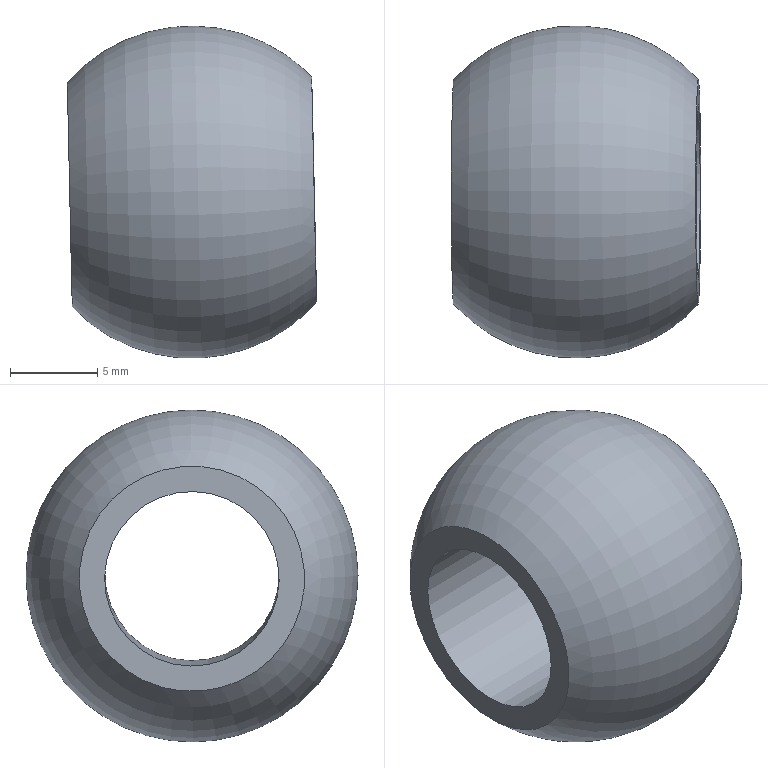Part | NX | features 2 2 | 1 solid | 4 faces | box 14.279 x 19.031 x 19.031 mm | volume 2165 mm3 | plane 2 | cylinder 1 | torus 1 | commonest cylinder face diameters 10 x1
STEP:
#1=CARTESIAN_POINT('',(11.562,55.788,-650.48));
#2=VERTEX_POINT('',#1);
#3=CARTESIAN_POINT('',(11.498,51.587,-647.769));
#4=DIRECTION('',(-0.9998,0.0009413,-0.0219));
#5=DIRECTION('',(0.01267,0.8402,-0.5422));
#6=AXIS2_PLACEMENT_3D('',#3,#4,#5);
#7=CIRCLE('',#6,5.);
#8=EDGE_CURVE('',#2,#2,#7,.T.);
#9=ORIENTED_EDGE('',*,*,#8,.F.);
#10=EDGE_LOOP('',(#9));
#11=FACE_BOUND('',#10,.T.);
#12=CARTESIAN_POINT('',(-2.435,55.801,-650.786));
#13=VERTEX_POINT('',#12);
#14=CARTESIAN_POINT('',(-2.498,51.6,-648.076));
#15=DIRECTION('',(0.9998,-0.0009413,0.0219));
#16=DIRECTION('',(0.01267,0.8402,-0.5422));
#17=AXIS2_PLACEMENT_3D('',#14,#15,#16);
#18=CIRCLE('',#17,5.);
#19=EDGE_CURVE('',#13,#13,#18,.T.);
#20=ORIENTED_EDGE('',*,*,#19,.F.);
#21=EDGE_LOOP('',(#20));
#22=FACE_BOUND('',#21,.T.);
#23=CARTESIAN_POINT('',(4.5,51.593,-647.922));
#24=DIRECTION('',(-0.9998,0.0009413,-0.0219));
#25=DIRECTION('',(0.01267,0.8402,-0.5422));
#26=AXIS2_PLACEMENT_3D('',#23,#24,#25);
#27=CYLINDRICAL_SURFACE('',#26,5.);
#28=ADVANCED_FACE('',(#11,#22),#27,.F.);
#29=ORIENTED_EDGE('',*,*,#19,.T.);
#30=EDGE_LOOP('',(#29));
#31=FACE_BOUND('',#30,.T.);
#32=CARTESIAN_POINT('',(-2.433,57.453,-650.785));
#33=VERTEX_POINT('',#32);
#34=CARTESIAN_POINT('',(-2.498,51.6,-648.076));
#35=DIRECTION('',(-0.9998,0.0009413,-0.0219));
#36=DIRECTION('',(0.01006,0.9075,-0.42));
#37=AXIS2_PLACEMENT_3D('',#34,#35,#36);
#38=CIRCLE('',#37,6.45);
#39=EDGE_CURVE('',#33,#33,#38,.T.);
#40=ORIENTED_EDGE('',*,*,#39,.T.);
#41=EDGE_LOOP('',(#40));
#42=FACE_BOUND('',#41,.T.);
#43=CARTESIAN_POINT('',(-2.61,54.005,-642.882));
#44=DIRECTION('',(-0.9998,0.0009413,-0.0219));
#45=DIRECTION('',(0.01267,0.8402,-0.5422));
#46=AXIS2_PLACEMENT_3D('',#43,#44,#45);
#47=PLANE('',#46);
#48=ADVANCED_FACE('',(#31,#42),#47,.T.);
#49=ORIENTED_EDGE('',*,*,#8,.T.);
#50=EDGE_LOOP('',(#49));
#51=FACE_BOUND('',#50,.T.);
#52=CARTESIAN_POINT('',(11.58,57.006,-651.266));
#53=VERTEX_POINT('',#52);
#54=CARTESIAN_POINT('',(11.498,51.587,-647.769));
#55=DIRECTION('',(0.9998,-0.0009413,0.0219));
#56=DIRECTION('',(0.01267,0.8402,-0.5422));
#57=AXIS2_PLACEMENT_3D('',#54,#55,#56);
#58=CIRCLE('',#57,6.45);
#59=EDGE_CURVE('',#53,#53,#58,.T.);
#60=ORIENTED_EDGE('',*,*,#59,.T.);
#61=EDGE_LOOP('',(#60));
#62=FACE_BOUND('',#61,.T.);
#63=CARTESIAN_POINT('',(11.387,53.992,-642.575));
#64=DIRECTION('',(0.9998,-0.0009413,0.0219));
#65=DIRECTION('',(-0.01267,-0.8402,0.5422));
#66=AXIS2_PLACEMENT_3D('',#63,#64,#65);
#67=PLANE('',#66);
#68=ADVANCED_FACE('',(#51,#62),#67,.T.);
#69=ORIENTED_EDGE('',*,*,#39,.F.);
#70=EDGE_LOOP('',(#69));
#71=FACE_BOUND('',#70,.T.);
#72=ORIENTED_EDGE('',*,*,#59,.F.);
#73=EDGE_LOOP('',(#72));
#74=FACE_BOUND('',#73,.T.);
#75=CARTESIAN_POINT('',(4.5,51.593,-647.922));
#76=DIRECTION('',(-0.9998,0.0009413,-0.0219));
#77=DIRECTION('',(-0.01006,-0.9075,0.42));
#78=AXIS2_PLACEMENT_3D('',#75,#76,#77);
#79=DEGENERATE_TOROIDAL_SURFACE('',#78,0.009538,9.525,.F.);
#80=ADVANCED_FACE('',(#71,#74),#79,.F.);
#81=CLOSED_SHELL('',(#28,#48,#68,#80));
#82=MANIFOLD_SOLID_BREP('',#81);
#83=(LENGTH_UNIT()NAMED_UNIT(*)SI_UNIT(.MILLI.,.METRE.));
#84=UNCERTAINTY_MEASURE_WITH_UNIT(LENGTH_MEASURE(0.00001),#83,'','');
#85=(NAMED_UNIT(*)PLANE_ANGLE_UNIT()SI_UNIT($,.RADIAN.));
#86=(NAMED_UNIT(*)SI_UNIT($,.STERADIAN.)SOLID_ANGLE_UNIT());
#87=(GEOMETRIC_REPRESENTATION_CONTEXT(3)GLOBAL_UNCERTAINTY_ASSIGNED_CONTEXT((#84))GLOBAL_UNIT_ASSIGNED_CONTEXT((#83,#85,#86))REPRESENTATION_CONTEXT('',''));
#88=ADVANCED_BREP_SHAPE_REPRESENTATION('',(#82),#87);